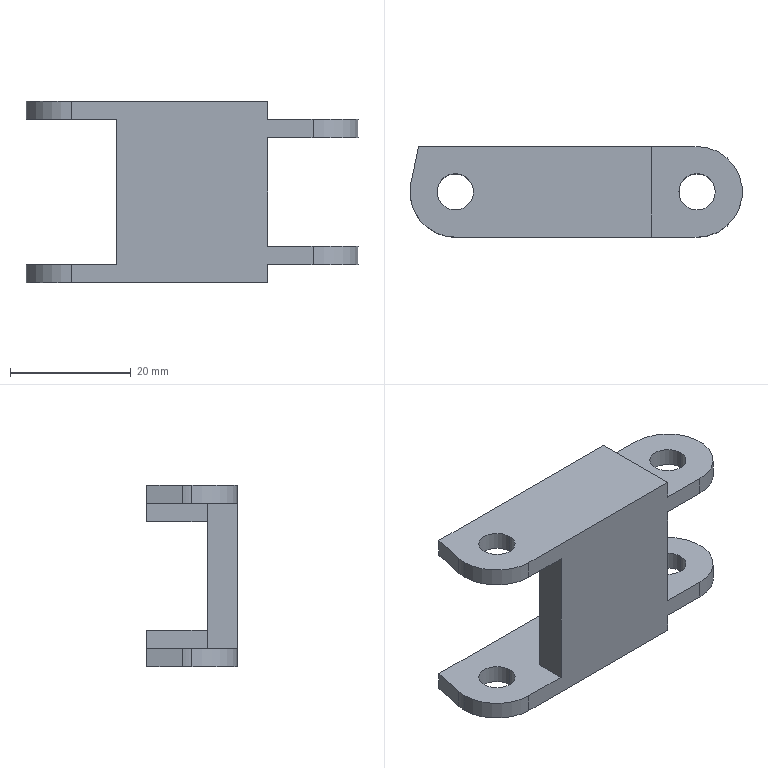Part | SolidWorks | features ICE 3, Extrusion 1 | 1 solid | 34 faces | box 55 x 15 x 30 mm | volume 7665 mm3 | plane 20 | cylinder 14 | commonest cylinder face diameters 6 x8 15 x6
STEP:
#1=CARTESIAN_POINT('',(12.262,7.5,3.));
#2=VERTEX_POINT('',#1);
#3=CARTESIAN_POINT('',(6.262,7.5,3.));
#4=VERTEX_POINT('',#3);
#5=CARTESIAN_POINT('',(9.262,7.5,3.));
#6=DIRECTION('',(0.,0.,-1.));
#7=DIRECTION('',(-1.,0.,0.));
#8=AXIS2_PLACEMENT_3D('',#5,#6,#7);
#9=CIRCLE('',#8,3.);
#10=EDGE_CURVE('',#2,#4,#9,.T.);
#11=ORIENTED_EDGE('',*,*,#10,.F.);
#12=CARTESIAN_POINT('',(12.262,7.5,0.));
#13=VERTEX_POINT('',#12);
#14=CARTESIAN_POINT('',(12.262,7.5,30.));
#15=DIRECTION('',(0.,0.,-1.));
#16=VECTOR('',#15,1000.);
#17=LINE('',#14,#16);
#18=EDGE_CURVE('',#2,#13,#17,.T.);
#19=ORIENTED_EDGE('',*,*,#18,.T.);
#20=CARTESIAN_POINT('',(6.262,7.5,0.));
#21=VERTEX_POINT('',#20);
#22=CARTESIAN_POINT('',(9.262,7.5,0.));
#23=DIRECTION('',(0.,0.,1.));
#24=DIRECTION('',(1.,0.,0.));
#25=AXIS2_PLACEMENT_3D('',#22,#23,#24);
#26=CIRCLE('',#25,3.);
#27=EDGE_CURVE('',#21,#13,#26,.T.);
#28=ORIENTED_EDGE('',*,*,#27,.F.);
#29=CARTESIAN_POINT('',(6.262,7.5,30.));
#30=DIRECTION('',(0.,0.,-1.));
#31=VECTOR('',#30,1000.);
#32=LINE('',#29,#31);
#33=EDGE_CURVE('',#4,#21,#32,.T.);
#34=ORIENTED_EDGE('',*,*,#33,.F.);
#35=EDGE_LOOP('',(#11,#19,#28,#34));
#36=FACE_OUTER_BOUND('',#35,.T.);
#37=CARTESIAN_POINT('',(9.262,7.5,30.));
#38=DIRECTION('',(0.,0.,-1.));
#39=DIRECTION('',(-1.,0.,0.));
#40=AXIS2_PLACEMENT_3D('',#37,#38,#39);
#41=CYLINDRICAL_SURFACE('',#40,3.);
#42=ADVANCED_FACE('',(#36),#41,.F.);
#43=CARTESIAN_POINT('',(9.262,0.,3.));
#44=VERTEX_POINT('',#43);
#45=CARTESIAN_POINT('',(1.762,7.5,3.));
#46=VERTEX_POINT('',#45);
#47=CARTESIAN_POINT('',(9.262,7.5,3.));
#48=DIRECTION('',(0.,0.,-1.));
#49=DIRECTION('',(-1.,0.,0.));
#50=AXIS2_PLACEMENT_3D('',#47,#48,#49);
#51=CIRCLE('',#50,7.5);
#52=EDGE_CURVE('',#44,#46,#51,.T.);
#53=ORIENTED_EDGE('',*,*,#52,.T.);
#54=CARTESIAN_POINT('',(1.762,7.5,0.));
#55=VERTEX_POINT('',#54);
#56=CARTESIAN_POINT('',(1.762,7.5,30.));
#57=DIRECTION('',(0.,0.,-1.));
#58=VECTOR('',#57,1000.);
#59=LINE('',#56,#58);
#60=EDGE_CURVE('',#46,#55,#59,.T.);
#61=ORIENTED_EDGE('',*,*,#60,.T.);
#62=CARTESIAN_POINT('',(9.262,0.,0.));
#63=VERTEX_POINT('',#62);
#64=CARTESIAN_POINT('',(9.262,7.5,0.));
#65=DIRECTION('',(0.,0.,1.));
#66=DIRECTION('',(1.,0.,0.));
#67=AXIS2_PLACEMENT_3D('',#64,#65,#66);
#68=CIRCLE('',#67,7.5);
#69=EDGE_CURVE('',#55,#63,#68,.T.);
#70=ORIENTED_EDGE('',*,*,#69,.T.);
#71=CARTESIAN_POINT('',(9.262,0.,30.));
#72=DIRECTION('',(0.,0.,-1.));
#73=VECTOR('',#72,1000.);
#74=LINE('',#71,#73);
#75=EDGE_CURVE('',#44,#63,#74,.T.);
#76=ORIENTED_EDGE('',*,*,#75,.F.);
#77=EDGE_LOOP('',(#53,#61,#70,#76));
#78=FACE_OUTER_BOUND('',#77,.T.);
#79=CARTESIAN_POINT('',(9.262,7.5,30.));
#80=DIRECTION('',(0.,0.,-1.));
#81=DIRECTION('',(-1.,0.,0.));
#82=AXIS2_PLACEMENT_3D('',#79,#80,#81);
#83=CYLINDRICAL_SURFACE('',#82,7.5);
#84=ADVANCED_FACE('',(#78),#83,.T.);
#85=CARTESIAN_POINT('',(6.262,7.5,30.));
#86=VERTEX_POINT('',#85);
#87=CARTESIAN_POINT('',(12.262,7.5,30.));
#88=VERTEX_POINT('',#87);
#89=CARTESIAN_POINT('',(9.262,7.5,30.));
#90=DIRECTION('',(0.,0.,1.));
#91=DIRECTION('',(1.,0.,0.));
#92=AXIS2_PLACEMENT_3D('',#89,#90,#91);
#93=CIRCLE('',#92,3.);
#94=EDGE_CURVE('',#86,#88,#93,.T.);
#95=ORIENTED_EDGE('',*,*,#94,.T.);
#96=CARTESIAN_POINT('',(12.262,7.5,27.));
#97=VERTEX_POINT('',#96);
#98=CARTESIAN_POINT('',(12.262,7.5,30.));
#99=DIRECTION('',(0.,0.,-1.));
#100=VECTOR('',#99,1000.);
#101=LINE('',#98,#100);
#102=EDGE_CURVE('',#88,#97,#101,.T.);
#103=ORIENTED_EDGE('',*,*,#102,.T.);
#104=CARTESIAN_POINT('',(6.262,7.5,27.));
#105=VERTEX_POINT('',#104);
#106=CARTESIAN_POINT('',(9.262,7.5,27.));
#107=DIRECTION('',(0.,0.,1.));
#108=DIRECTION('',(1.,0.,0.));
#109=AXIS2_PLACEMENT_3D('',#106,#107,#108);
#110=CIRCLE('',#109,3.);
#111=EDGE_CURVE('',#105,#97,#110,.T.);
#112=ORIENTED_EDGE('',*,*,#111,.F.);
#113=CARTESIAN_POINT('',(6.262,7.5,30.));
#114=DIRECTION('',(0.,0.,-1.));
#115=VECTOR('',#114,1000.);
#116=LINE('',#113,#115);
#117=EDGE_CURVE('',#86,#105,#116,.T.);
#118=ORIENTED_EDGE('',*,*,#117,.F.);
#119=EDGE_LOOP('',(#95,#103,#112,#118));
#120=FACE_OUTER_BOUND('',#119,.T.);
#121=CARTESIAN_POINT('',(9.262,7.5,30.));
#122=DIRECTION('',(0.,0.,-1.));
#123=DIRECTION('',(-1.,0.,0.));
#124=AXIS2_PLACEMENT_3D('',#121,#122,#123);
#125=CYLINDRICAL_SURFACE('',#124,3.);
#126=ADVANCED_FACE('',(#120),#125,.F.);
#127=CARTESIAN_POINT('',(1.762,7.5,30.));
#128=VERTEX_POINT('',#127);
#129=CARTESIAN_POINT('',(9.262,0.,30.));
#130=VERTEX_POINT('',#129);
#131=CARTESIAN_POINT('',(9.262,7.5,30.));
#132=DIRECTION('',(0.,0.,1.));
#133=DIRECTION('',(1.,0.,0.));
#134=AXIS2_PLACEMENT_3D('',#131,#132,#133);
#135=CIRCLE('',#134,7.5);
#136=EDGE_CURVE('',#128,#130,#135,.T.);
#137=ORIENTED_EDGE('',*,*,#136,.F.);
#138=CARTESIAN_POINT('',(1.762,7.5,27.));
#139=VERTEX_POINT('',#138);
#140=CARTESIAN_POINT('',(1.762,7.5,30.));
#141=DIRECTION('',(0.,0.,-1.));
#142=VECTOR('',#141,1000.);
#143=LINE('',#140,#142);
#144=EDGE_CURVE('',#128,#139,#143,.T.);
#145=ORIENTED_EDGE('',*,*,#144,.T.);
#146=CARTESIAN_POINT('',(9.262,0.,27.));
#147=VERTEX_POINT('',#146);
#148=CARTESIAN_POINT('',(9.262,7.5,27.));
#149=DIRECTION('',(0.,0.,1.));
#150=DIRECTION('',(1.,0.,0.));
#151=AXIS2_PLACEMENT_3D('',#148,#149,#150);
#152=CIRCLE('',#151,7.5);
#153=EDGE_CURVE('',#139,#147,#152,.T.);
#154=ORIENTED_EDGE('',*,*,#153,.T.);
#155=CARTESIAN_POINT('',(9.262,0.,30.));
#156=DIRECTION('',(0.,0.,-1.));
#157=VECTOR('',#156,1000.);
#158=LINE('',#155,#157);
#159=EDGE_CURVE('',#130,#147,#158,.T.);
#160=ORIENTED_EDGE('',*,*,#159,.F.);
#161=EDGE_LOOP('',(#137,#145,#154,#160));
#162=FACE_OUTER_BOUND('',#161,.T.);
#163=CARTESIAN_POINT('',(9.262,7.5,30.));
#164=DIRECTION('',(0.,0.,-1.));
#165=DIRECTION('',(-1.,0.,0.));
#166=AXIS2_PLACEMENT_3D('',#163,#164,#165);
#167=CYLINDRICAL_SURFACE('',#166,7.5);
#168=ADVANCED_FACE('',(#162),#167,.T.);
#169=CARTESIAN_POINT('',(52.262,7.5,27.));
#170=VERTEX_POINT('',#169);
#171=CARTESIAN_POINT('',(46.262,7.5,27.));
#172=VERTEX_POINT('',#171);
#173=CARTESIAN_POINT('',(49.262,7.5,27.));
#174=DIRECTION('',(0.,0.,-1.));
#175=DIRECTION('',(-1.,0.,0.));
#176=AXIS2_PLACEMENT_3D('',#173,#174,#175);
#177=CIRCLE('',#176,3.);
#178=EDGE_CURVE('',#170,#172,#177,.T.);
#179=ORIENTED_EDGE('',*,*,#178,.F.);
#180=CARTESIAN_POINT('',(52.262,7.5,24.));
#181=VERTEX_POINT('',#180);
#182=CARTESIAN_POINT('',(52.262,7.5,30.));
#183=DIRECTION('',(0.,0.,-1.));
#184=VECTOR('',#183,1000.);
#185=LINE('',#182,#184);
#186=EDGE_CURVE('',#170,#181,#185,.T.);
#187=ORIENTED_EDGE('',*,*,#186,.T.);
#188=CARTESIAN_POINT('',(46.262,7.5,24.));
#189=VERTEX_POINT('',#188);
#190=CARTESIAN_POINT('',(49.262,7.5,24.));
#191=DIRECTION('',(0.,0.,1.));
#192=DIRECTION('',(1.,0.,0.));
#193=AXIS2_PLACEMENT_3D('',#190,#191,#192);
#194=CIRCLE('',#193,3.);
#195=EDGE_CURVE('',#189,#181,#194,.T.);
#196=ORIENTED_EDGE('',*,*,#195,.F.);
#197=CARTESIAN_POINT('',(46.262,7.5,30.));
#198=DIRECTION('',(0.,0.,-1.));
#199=VECTOR('',#198,1000.);
#200=LINE('',#197,#199);
#201=EDGE_CURVE('',#172,#189,#200,.T.);
#202=ORIENTED_EDGE('',*,*,#201,.F.);
#203=EDGE_LOOP('',(#179,#187,#196,#202));
#204=FACE_OUTER_BOUND('',#203,.T.);
#205=CARTESIAN_POINT('',(49.262,7.5,30.));
#206=DIRECTION('',(0.,0.,-1.));
#207=DIRECTION('',(-1.,0.,0.));
#208=AXIS2_PLACEMENT_3D('',#205,#206,#207);
#209=CYLINDRICAL_SURFACE('',#208,3.);
#210=ADVANCED_FACE('',(#204),#209,.F.);
#211=CARTESIAN_POINT('',(52.262,7.5,6.));
#212=VERTEX_POINT('',#211);
#213=CARTESIAN_POINT('',(46.262,7.5,6.));
#214=VERTEX_POINT('',#213);
#215=CARTESIAN_POINT('',(49.262,7.5,6.));
#216=DIRECTION('',(0.,0.,-1.));
#217=DIRECTION('',(-1.,0.,0.));
#218=AXIS2_PLACEMENT_3D('',#215,#216,#217);
#219=CIRCLE('',#218,3.);
#220=EDGE_CURVE('',#212,#214,#219,.T.);
#221=ORIENTED_EDGE('',*,*,#220,.F.);
#222=CARTESIAN_POINT('',(52.262,7.5,3.));
#223=VERTEX_POINT('',#222);
#224=CARTESIAN_POINT('',(52.262,7.5,30.));
#225=DIRECTION('',(0.,0.,-1.));
#226=VECTOR('',#225,1000.);
#227=LINE('',#224,#226);
#228=EDGE_CURVE('',#212,#223,#227,.T.);
#229=ORIENTED_EDGE('',*,*,#228,.T.);
#230=CARTESIAN_POINT('',(46.262,7.5,3.));
#231=VERTEX_POINT('',#230);
#232=CARTESIAN_POINT('',(49.262,7.5,3.));
#233=DIRECTION('',(0.,0.,1.));
#234=DIRECTION('',(1.,0.,0.));
#235=AXIS2_PLACEMENT_3D('',#232,#233,#234);
#236=CIRCLE('',#235,3.);
#237=EDGE_CURVE('',#231,#223,#236,.T.);
#238=ORIENTED_EDGE('',*,*,#237,.F.);
#239=CARTESIAN_POINT('',(46.262,7.5,30.));
#240=DIRECTION('',(0.,0.,-1.));
#241=VECTOR('',#240,1000.);
#242=LINE('',#239,#241);
#243=EDGE_CURVE('',#214,#231,#242,.T.);
#244=ORIENTED_EDGE('',*,*,#243,.F.);
#245=EDGE_LOOP('',(#221,#229,#238,#244));
#246=FACE_OUTER_BOUND('',#245,.T.);
#247=CARTESIAN_POINT('',(49.262,7.5,30.));
#248=DIRECTION('',(0.,0.,-1.));
#249=DIRECTION('',(-1.,0.,0.));
#250=AXIS2_PLACEMENT_3D('',#247,#248,#249);
#251=CYLINDRICAL_SURFACE('',#250,3.);
#252=ADVANCED_FACE('',(#246),#251,.F.);
#253=ORIENTED_EDGE('',*,*,#228,.F.);
#254=CARTESIAN_POINT('',(49.262,7.5,6.));
#255=DIRECTION('',(0.,0.,-1.));
#256=DIRECTION('',(-1.,0.,0.));
#257=AXIS2_PLACEMENT_3D('',#254,#255,#256);
#258=CIRCLE('',#257,3.);
#259=EDGE_CURVE('',#214,#212,#258,.T.);
#260=ORIENTED_EDGE('',*,*,#259,.F.);
#261=ORIENTED_EDGE('',*,*,#243,.T.);
#262=CARTESIAN_POINT('',(49.262,7.5,3.));
#263=DIRECTION('',(0.,0.,1.));
#264=DIRECTION('',(1.,0.,0.));
#265=AXIS2_PLACEMENT_3D('',#262,#263,#264);
#266=CIRCLE('',#265,3.);
#267=EDGE_CURVE('',#223,#231,#266,.T.);
#268=ORIENTED_EDGE('',*,*,#267,.F.);
#269=EDGE_LOOP('',(#253,#260,#261,#268));
#270=FACE_OUTER_BOUND('',#269,.T.);
#271=CARTESIAN_POINT('',(49.262,7.5,30.));
#272=DIRECTION('',(0.,0.,-1.));
#273=DIRECTION('',(-1.,0.,0.));
#274=AXIS2_PLACEMENT_3D('',#271,#272,#273);
#275=CYLINDRICAL_SURFACE('',#274,3.);
#276=ADVANCED_FACE('',(#270),#275,.F.);
#277=CARTESIAN_POINT('',(49.262,15.,6.));
#278=VERTEX_POINT('',#277);
#279=CARTESIAN_POINT('',(49.262,0.,6.));
#280=VERTEX_POINT('',#279);
#281=CARTESIAN_POINT('',(49.262,7.5,6.));
#282=DIRECTION('',(0.,0.,-1.));
#283=DIRECTION('',(-1.,0.,0.));
#284=AXIS2_PLACEMENT_3D('',#281,#282,#283);
#285=CIRCLE('',#284,7.5);
#286=EDGE_CURVE('',#278,#280,#285,.T.);
#287=ORIENTED_EDGE('',*,*,#286,.T.);
#288=CARTESIAN_POINT('',(49.262,0.,3.));
#289=VERTEX_POINT('',#288);
#290=CARTESIAN_POINT('',(49.262,0.,30.));
#291=DIRECTION('',(0.,0.,-1.));
#292=VECTOR('',#291,1000.);
#293=LINE('',#290,#292);
#294=EDGE_CURVE('',#280,#289,#293,.T.);
#295=ORIENTED_EDGE('',*,*,#294,.T.);
#296=CARTESIAN_POINT('',(49.262,15.,3.));
#297=VERTEX_POINT('',#296);
#298=CARTESIAN_POINT('',(49.262,7.5,3.));
#299=DIRECTION('',(0.,0.,1.));
#300=DIRECTION('',(1.,0.,0.));
#301=AXIS2_PLACEMENT_3D('',#298,#299,#300);
#302=CIRCLE('',#301,7.5);
#303=EDGE_CURVE('',#289,#297,#302,.T.);
#304=ORIENTED_EDGE('',*,*,#303,.T.);
#305=CARTESIAN_POINT('',(49.262,15.,30.));
#306=DIRECTION('',(0.,0.,-1.));
#307=VECTOR('',#306,1000.);
#308=LINE('',#305,#307);
#309=EDGE_CURVE('',#278,#297,#308,.T.);
#310=ORIENTED_EDGE('',*,*,#309,.F.);
#311=EDGE_LOOP('',(#287,#295,#304,#310));
#312=FACE_OUTER_BOUND('',#311,.T.);
#313=CARTESIAN_POINT('',(49.262,7.5,30.));
#314=DIRECTION('',(0.,0.,-1.));
#315=DIRECTION('',(-1.,0.,0.));
#316=AXIS2_PLACEMENT_3D('',#313,#314,#315);
#317=CYLINDRICAL_SURFACE('',#316,7.5);
#318=ADVANCED_FACE('',(#312),#317,.T.);
#319=CARTESIAN_POINT('',(36.762,15.,3.));
#320=VERTEX_POINT('',#319);
#321=CARTESIAN_POINT('',(3.188,15.,3.));
#322=VERTEX_POINT('',#321);
#323=CARTESIAN_POINT('',(-13.238,15.,3.));
#324=DIRECTION('',(-1.,0.,0.));
#325=VECTOR('',#324,1000.);
#326=LINE('',#323,#325);
#327=EDGE_CURVE('',#320,#322,#326,.T.);
#328=ORIENTED_EDGE('',*,*,#327,.F.);
#329=CARTESIAN_POINT('',(36.762,15.,6.));
#330=VERTEX_POINT('',#329);
#331=CARTESIAN_POINT('',(36.762,15.,3.));
#332=DIRECTION('',(0.,0.,-1.));
#333=VECTOR('',#332,1000.);
#334=LINE('',#331,#333);
#335=EDGE_CURVE('',#330,#320,#334,.T.);
#336=ORIENTED_EDGE('',*,*,#335,.F.);
#337=CARTESIAN_POINT('',(36.762,15.,6.));
#338=DIRECTION('',(-1.,0.,0.));
#339=VECTOR('',#338,1000.);
#340=LINE('',#337,#339);
#341=EDGE_CURVE('',#278,#330,#340,.T.);
#342=ORIENTED_EDGE('',*,*,#341,.F.);
#343=ORIENTED_EDGE('',*,*,#309,.T.);
#344=CARTESIAN_POINT('',(41.762,15.,3.));
#345=VERTEX_POINT('',#344);
#346=CARTESIAN_POINT('',(41.762,15.,3.));
#347=DIRECTION('',(1.,0.,0.));
#348=VECTOR('',#347,1000.);
#349=LINE('',#346,#348);
#350=EDGE_CURVE('',#345,#297,#349,.T.);
#351=ORIENTED_EDGE('',*,*,#350,.F.);
#352=CARTESIAN_POINT('',(41.762,15.,0.));
#353=VERTEX_POINT('',#352);
#354=CARTESIAN_POINT('',(41.762,15.,-3.));
#355=DIRECTION('',(0.,0.,1.));
#356=VECTOR('',#355,1000.);
#357=LINE('',#354,#356);
#358=EDGE_CURVE('',#353,#345,#357,.T.);
#359=ORIENTED_EDGE('',*,*,#358,.F.);
#360=CARTESIAN_POINT('',(3.188,15.,0.));
#361=VERTEX_POINT('',#360);
#362=CARTESIAN_POINT('',(3.188,15.,0.));
#363=DIRECTION('',(-1.,0.,0.));
#364=VECTOR('',#363,1000.);
#365=LINE('',#362,#364);
#366=EDGE_CURVE('',#353,#361,#365,.T.);
#367=ORIENTED_EDGE('',*,*,#366,.T.);
#368=CARTESIAN_POINT('',(3.188,15.,30.));
#369=DIRECTION('',(0.,0.,-1.));
#370=VECTOR('',#369,1000.);
#371=LINE('',#368,#370);
#372=EDGE_CURVE('',#322,#361,#371,.T.);
#373=ORIENTED_EDGE('',*,*,#372,.F.);
#374=EDGE_LOOP('',(#328,#336,#342,#343,#351,#359,#367,#373));
#375=FACE_OUTER_BOUND('',#374,.T.);
#376=CARTESIAN_POINT('',(3.188,15.,30.));
#377=DIRECTION('',(0.,-1.,0.));
#378=DIRECTION('',(0.,0.,-1.));
#379=AXIS2_PLACEMENT_3D('',#376,#377,#378);
#380=PLANE('',#379);
#381=ADVANCED_FACE('',(#375),#380,.F.);
#382=CARTESIAN_POINT('',(16.762,5.,3.));
#383=VERTEX_POINT('',#382);
#384=CARTESIAN_POINT('',(16.762,5.,27.));
#385=VERTEX_POINT('',#384);
#386=CARTESIAN_POINT('',(16.762,5.,3.));
#387=DIRECTION('',(0.,0.,1.));
#388=VECTOR('',#387,1000.);
#389=LINE('',#386,#388);
#390=EDGE_CURVE('',#383,#385,#389,.T.);
#391=ORIENTED_EDGE('',*,*,#390,.F.);
#392=CARTESIAN_POINT('',(16.762,0.,3.));
#393=VERTEX_POINT('',#392);
#394=CARTESIAN_POINT('',(16.762,-15.,3.));
#395=DIRECTION('',(0.,1.,0.));
#396=VECTOR('',#395,1000.);
#397=LINE('',#394,#396);
#398=EDGE_CURVE('',#393,#383,#397,.T.);
#399=ORIENTED_EDGE('',*,*,#398,.F.);
#400=CARTESIAN_POINT('',(16.762,0.,27.));
#401=VERTEX_POINT('',#400);
#402=CARTESIAN_POINT('',(16.762,0.,30.));
#403=DIRECTION('',(0.,0.,-1.));
#404=VECTOR('',#403,1000.);
#405=LINE('',#402,#404);
#406=EDGE_CURVE('',#401,#393,#405,.T.);
#407=ORIENTED_EDGE('',*,*,#406,.F.);
#408=CARTESIAN_POINT('',(16.762,-15.,27.));
#409=DIRECTION('',(0.,1.,0.));
#410=VECTOR('',#409,1000.);
#411=LINE('',#408,#410);
#412=EDGE_CURVE('',#401,#385,#411,.T.);
#413=ORIENTED_EDGE('',*,*,#412,.T.);
#414=EDGE_LOOP('',(#391,#399,#407,#413));
#415=FACE_OUTER_BOUND('',#414,.T.);
#416=CARTESIAN_POINT('',(16.762,-15.,3.));
#417=DIRECTION('',(1.,0.,0.));
#418=DIRECTION('',(0.,0.,-1.));
#419=AXIS2_PLACEMENT_3D('',#416,#417,#418);
#420=PLANE('',#419);
#421=ADVANCED_FACE('',(#415),#420,.F.);
#422=ORIENTED_EDGE('',*,*,#186,.F.);
#423=CARTESIAN_POINT('',(49.262,7.5,27.));
#424=DIRECTION('',(0.,0.,-1.));
#425=DIRECTION('',(-1.,0.,0.));
#426=AXIS2_PLACEMENT_3D('',#423,#424,#425);
#427=CIRCLE('',#426,3.);
#428=EDGE_CURVE('',#172,#170,#427,.T.);
#429=ORIENTED_EDGE('',*,*,#428,.F.);
#430=ORIENTED_EDGE('',*,*,#201,.T.);
#431=CARTESIAN_POINT('',(49.262,7.5,24.));
#432=DIRECTION('',(0.,0.,1.));
#433=DIRECTION('',(1.,0.,0.));
#434=AXIS2_PLACEMENT_3D('',#431,#432,#433);
#435=CIRCLE('',#434,3.);
#436=EDGE_CURVE('',#181,#189,#435,.T.);
#437=ORIENTED_EDGE('',*,*,#436,.F.);
#438=EDGE_LOOP('',(#422,#429,#430,#437));
#439=FACE_OUTER_BOUND('',#438,.T.);
#440=CARTESIAN_POINT('',(49.262,7.5,30.));
#441=DIRECTION('',(0.,0.,-1.));
#442=DIRECTION('',(-1.,0.,0.));
#443=AXIS2_PLACEMENT_3D('',#440,#441,#442);
#444=CYLINDRICAL_SURFACE('',#443,3.);
#445=ADVANCED_FACE('',(#439),#444,.F.);
#446=CARTESIAN_POINT('',(3.188,15.,30.));
#447=VERTEX_POINT('',#446);
#448=CARTESIAN_POINT('',(3.188,15.,27.));
#449=VERTEX_POINT('',#448);
#450=CARTESIAN_POINT('',(3.188,15.,30.));
#451=DIRECTION('',(0.,0.,-1.));
#452=VECTOR('',#451,1000.);
#453=LINE('',#450,#452);
#454=EDGE_CURVE('',#447,#449,#453,.T.);
#455=ORIENTED_EDGE('',*,*,#454,.T.);
#456=CARTESIAN_POINT('',(1.926,9.059,27.));
#457=VERTEX_POINT('',#456);
#458=CARTESIAN_POINT('',(1.926,9.059,27.));
#459=DIRECTION('',(-0.2079,-0.9781,0.));
#460=VECTOR('',#459,1000.);
#461=LINE('',#458,#460);
#462=EDGE_CURVE('',#449,#457,#461,.T.);
#463=ORIENTED_EDGE('',*,*,#462,.T.);
#464=CARTESIAN_POINT('',(1.926,9.059,30.));
#465=VERTEX_POINT('',#464);
#466=CARTESIAN_POINT('',(1.926,9.059,30.));
#467=DIRECTION('',(0.,0.,-1.));
#468=VECTOR('',#467,1000.);
#469=LINE('',#466,#468);
#470=EDGE_CURVE('',#465,#457,#469,.T.);
#471=ORIENTED_EDGE('',*,*,#470,.F.);
#472=CARTESIAN_POINT('',(1.926,9.059,30.));
#473=DIRECTION('',(-0.2079,-0.9781,0.));
#474=VECTOR('',#473,1000.);
#475=LINE('',#472,#474);
#476=EDGE_CURVE('',#447,#465,#475,.T.);
#477=ORIENTED_EDGE('',*,*,#476,.F.);
#478=EDGE_LOOP('',(#455,#463,#471,#477));
#479=FACE_OUTER_BOUND('',#478,.T.);
#480=CARTESIAN_POINT('',(1.926,9.059,30.));
#481=DIRECTION('',(0.9781,-0.2079,0.));
#482=DIRECTION('',(0.2079,0.9781,0.));
#483=AXIS2_PLACEMENT_3D('',#480,#481,#482);
#484=PLANE('',#483);
#485=ADVANCED_FACE('',(#479),#484,.F.);
#486=ORIENTED_EDGE('',*,*,#144,.F.);
#487=CARTESIAN_POINT('',(9.262,7.5,30.));
#488=DIRECTION('',(0.,0.,1.));
#489=DIRECTION('',(1.,0.,0.));
#490=AXIS2_PLACEMENT_3D('',#487,#488,#489);
#491=CIRCLE('',#490,7.5);
#492=EDGE_CURVE('',#465,#128,#491,.T.);
#493=ORIENTED_EDGE('',*,*,#492,.F.);
#494=ORIENTED_EDGE('',*,*,#470,.T.);
#495=CARTESIAN_POINT('',(9.262,7.5,27.));
#496=DIRECTION('',(0.,0.,1.));
#497=DIRECTION('',(1.,0.,0.));
#498=AXIS2_PLACEMENT_3D('',#495,#496,#497);
#499=CIRCLE('',#498,7.5);
#500=EDGE_CURVE('',#457,#139,#499,.T.);
#501=ORIENTED_EDGE('',*,*,#500,.T.);
#502=EDGE_LOOP('',(#486,#493,#494,#501));
#503=FACE_OUTER_BOUND('',#502,.T.);
#504=CARTESIAN_POINT('',(9.262,7.5,30.));
#505=DIRECTION('',(0.,0.,-1.));
#506=DIRECTION('',(-1.,0.,0.));
#507=AXIS2_PLACEMENT_3D('',#504,#505,#506);
#508=CYLINDRICAL_SURFACE('',#507,7.5);
#509=ADVANCED_FACE('',(#503),#508,.T.);
#510=ORIENTED_EDGE('',*,*,#102,.F.);
#511=CARTESIAN_POINT('',(9.262,7.5,30.));
#512=DIRECTION('',(0.,0.,1.));
#513=DIRECTION('',(1.,0.,0.));
#514=AXIS2_PLACEMENT_3D('',#511,#512,#513);
#515=CIRCLE('',#514,3.);
#516=EDGE_CURVE('',#88,#86,#515,.T.);
#517=ORIENTED_EDGE('',*,*,#516,.T.);
#518=ORIENTED_EDGE('',*,*,#117,.T.);
#519=CARTESIAN_POINT('',(9.262,7.5,27.));
#520=DIRECTION('',(0.,0.,1.));
#521=DIRECTION('',(1.,0.,0.));
#522=AXIS2_PLACEMENT_3D('',#519,#520,#521);
#523=CIRCLE('',#522,3.);
#524=EDGE_CURVE('',#97,#105,#523,.T.);
#525=ORIENTED_EDGE('',*,*,#524,.F.);
#526=EDGE_LOOP('',(#510,#517,#518,#525));
#527=FACE_OUTER_BOUND('',#526,.T.);
#528=CARTESIAN_POINT('',(9.262,7.5,30.));
#529=DIRECTION('',(0.,0.,-1.));
#530=DIRECTION('',(-1.,0.,0.));
#531=AXIS2_PLACEMENT_3D('',#528,#529,#530);
#532=CYLINDRICAL_SURFACE('',#531,3.);
#533=ADVANCED_FACE('',(#527),#532,.F.);
#534=CARTESIAN_POINT('',(41.762,15.,30.));
#535=VERTEX_POINT('',#534);
#536=CARTESIAN_POINT('',(41.762,0.,30.));
#537=VERTEX_POINT('',#536);
#538=CARTESIAN_POINT('',(41.762,7.5,30.));
#539=DIRECTION('',(0.,-1.,0.));
#540=VECTOR('',#539,1000.);
#541=LINE('',#538,#540);
#542=EDGE_CURVE('',#535,#537,#541,.T.);
#543=ORIENTED_EDGE('',*,*,#542,.F.);
#544=CARTESIAN_POINT('',(3.188,15.,30.));
#545=DIRECTION('',(-1.,0.,0.));
#546=VECTOR('',#545,1000.);
#547=LINE('',#544,#546);
#548=EDGE_CURVE('',#535,#447,#547,.T.);
#549=ORIENTED_EDGE('',*,*,#548,.T.);
#550=ORIENTED_EDGE('',*,*,#476,.T.);
#551=ORIENTED_EDGE('',*,*,#492,.T.);
#552=ORIENTED_EDGE('',*,*,#136,.T.);
#553=CARTESIAN_POINT('',(49.262,0.,30.));
#554=DIRECTION('',(1.,0.,0.));
#555=VECTOR('',#554,1000.);
#556=LINE('',#553,#555);
#557=EDGE_CURVE('',#130,#537,#556,.T.);
#558=ORIENTED_EDGE('',*,*,#557,.T.);
#559=EDGE_LOOP('',(#543,#549,#550,#551,#552,#558));
#560=FACE_OUTER_BOUND('',#559,.T.);
#561=ORIENTED_EDGE('',*,*,#94,.F.);
#562=ORIENTED_EDGE('',*,*,#516,.F.);
#563=EDGE_LOOP('',(#561,#562));
#564=FACE_BOUND('',#563,.T.);
#565=CARTESIAN_POINT('',(49.262,7.5,30.));
#566=DIRECTION('',(0.,0.,1.));
#567=DIRECTION('',(1.,0.,0.));
#568=AXIS2_PLACEMENT_3D('',#565,#566,#567);
#569=PLANE('',#568);
#570=ADVANCED_FACE('',(#560,#564),#569,.T.);
#571=ORIENTED_EDGE('',*,*,#366,.F.);
#572=CARTESIAN_POINT('',(41.762,0.,0.));
#573=VERTEX_POINT('',#572);
#574=CARTESIAN_POINT('',(41.762,7.5,0.));
#575=DIRECTION('',(0.,-1.,0.));
#576=VECTOR('',#575,1000.);
#577=LINE('',#574,#576);
#578=EDGE_CURVE('',#353,#573,#577,.T.);
#579=ORIENTED_EDGE('',*,*,#578,.T.);
#580=CARTESIAN_POINT('',(49.262,0.,0.));
#581=DIRECTION('',(1.,0.,0.));
#582=VECTOR('',#581,1000.);
#583=LINE('',#580,#582);
#584=EDGE_CURVE('',#63,#573,#583,.T.);
#585=ORIENTED_EDGE('',*,*,#584,.F.);
#586=ORIENTED_EDGE('',*,*,#69,.F.);
#587=CARTESIAN_POINT('',(1.926,9.059,0.));
#588=VERTEX_POINT('',#587);
#589=CARTESIAN_POINT('',(9.262,7.5,0.));
#590=DIRECTION('',(0.,0.,1.));
#591=DIRECTION('',(1.,0.,0.));
#592=AXIS2_PLACEMENT_3D('',#589,#590,#591);
#593=CIRCLE('',#592,7.5);
#594=EDGE_CURVE('',#588,#55,#593,.T.);
#595=ORIENTED_EDGE('',*,*,#594,.F.);
#596=CARTESIAN_POINT('',(1.926,9.059,0.));
#597=DIRECTION('',(-0.2079,-0.9781,0.));
#598=VECTOR('',#597,1000.);
#599=LINE('',#596,#598);
#600=EDGE_CURVE('',#361,#588,#599,.T.);
#601=ORIENTED_EDGE('',*,*,#600,.F.);
#602=EDGE_LOOP('',(#571,#579,#585,#586,#595,#601));
#603=FACE_OUTER_BOUND('',#602,.T.);
#604=ORIENTED_EDGE('',*,*,#27,.T.);
#605=CARTESIAN_POINT('',(9.262,7.5,0.));
#606=DIRECTION('',(0.,0.,1.));
#607=DIRECTION('',(1.,0.,0.));
#608=AXIS2_PLACEMENT_3D('',#605,#606,#607);
#609=CIRCLE('',#608,3.);
#610=EDGE_CURVE('',#13,#21,#609,.T.);
#611=ORIENTED_EDGE('',*,*,#610,.T.);
#612=EDGE_LOOP('',(#604,#611));
#613=FACE_BOUND('',#612,.T.);
#614=CARTESIAN_POINT('',(49.262,7.5,0.));
#615=DIRECTION('',(0.,0.,1.));
#616=DIRECTION('',(1.,0.,0.));
#617=AXIS2_PLACEMENT_3D('',#614,#615,#616);
#618=PLANE('',#617);
#619=ADVANCED_FACE('',(#603,#613),#618,.F.);
#620=CARTESIAN_POINT('',(36.762,15.,27.));
#621=VERTEX_POINT('',#620);
#622=CARTESIAN_POINT('',(36.762,15.,24.));
#623=VERTEX_POINT('',#622);
#624=CARTESIAN_POINT('',(36.762,15.,24.));
#625=DIRECTION('',(0.,0.,-1.));
#626=VECTOR('',#625,1000.);
#627=LINE('',#624,#626);
#628=EDGE_CURVE('',#621,#623,#627,.T.);
#629=ORIENTED_EDGE('',*,*,#628,.F.);
#630=CARTESIAN_POINT('',(-13.238,15.,27.));
#631=DIRECTION('',(1.,0.,0.));
#632=VECTOR('',#631,1000.);
#633=LINE('',#630,#632);
#634=EDGE_CURVE('',#449,#621,#633,.T.);
#635=ORIENTED_EDGE('',*,*,#634,.F.);
#636=ORIENTED_EDGE('',*,*,#454,.F.);
#637=ORIENTED_EDGE('',*,*,#548,.F.);
#638=CARTESIAN_POINT('',(41.762,15.,27.));
#639=VERTEX_POINT('',#638);
#640=CARTESIAN_POINT('',(41.762,15.,27.));
#641=DIRECTION('',(0.,0.,1.));
#642=VECTOR('',#641,1000.);
#643=LINE('',#640,#642);
#644=EDGE_CURVE('',#639,#535,#643,.T.);
#645=ORIENTED_EDGE('',*,*,#644,.F.);
#646=CARTESIAN_POINT('',(49.262,15.,27.));
#647=VERTEX_POINT('',#646);
#648=CARTESIAN_POINT('',(41.762,15.,27.));
#649=DIRECTION('',(-1.,0.,0.));
#650=VECTOR('',#649,1000.);
#651=LINE('',#648,#650);
#652=EDGE_CURVE('',#647,#639,#651,.T.);
#653=ORIENTED_EDGE('',*,*,#652,.F.);
#654=CARTESIAN_POINT('',(49.262,15.,24.));
#655=VERTEX_POINT('',#654);
#656=CARTESIAN_POINT('',(49.262,15.,30.));
#657=DIRECTION('',(0.,0.,-1.));
#658=VECTOR('',#657,1000.);
#659=LINE('',#656,#658);
#660=EDGE_CURVE('',#647,#655,#659,.T.);
#661=ORIENTED_EDGE('',*,*,#660,.T.);
#662=CARTESIAN_POINT('',(36.762,15.,24.));
#663=DIRECTION('',(1.,0.,0.));
#664=VECTOR('',#663,1000.);
#665=LINE('',#662,#664);
#666=EDGE_CURVE('',#623,#655,#665,.T.);
#667=ORIENTED_EDGE('',*,*,#666,.F.);
#668=EDGE_LOOP('',(#629,#635,#636,#637,#645,#653,#661,#667));
#669=FACE_OUTER_BOUND('',#668,.T.);
#670=CARTESIAN_POINT('',(3.188,15.,30.));
#671=DIRECTION('',(0.,-1.,0.));
#672=DIRECTION('',(0.,0.,-1.));
#673=AXIS2_PLACEMENT_3D('',#670,#671,#672);
#674=PLANE('',#673);
#675=ADVANCED_FACE('',(#669),#674,.F.);
#676=CARTESIAN_POINT('',(1.926,9.059,3.));
#677=VERTEX_POINT('',#676);
#678=CARTESIAN_POINT('',(1.926,9.059,30.));
#679=DIRECTION('',(0.,0.,-1.));
#680=VECTOR('',#679,1000.);
#681=LINE('',#678,#680);
#682=EDGE_CURVE('',#677,#588,#681,.T.);
#683=ORIENTED_EDGE('',*,*,#682,.F.);
#684=CARTESIAN_POINT('',(1.926,9.059,3.));
#685=DIRECTION('',(0.2079,0.9781,0.));
#686=VECTOR('',#685,1000.);
#687=LINE('',#684,#686);
#688=EDGE_CURVE('',#677,#322,#687,.T.);
#689=ORIENTED_EDGE('',*,*,#688,.T.);
#690=ORIENTED_EDGE('',*,*,#372,.T.);
#691=ORIENTED_EDGE('',*,*,#600,.T.);
#692=EDGE_LOOP('',(#683,#689,#690,#691));
#693=FACE_OUTER_BOUND('',#692,.T.);
#694=CARTESIAN_POINT('',(1.926,9.059,30.));
#695=DIRECTION('',(0.9781,-0.2079,0.));
#696=DIRECTION('',(0.2079,0.9781,0.));
#697=AXIS2_PLACEMENT_3D('',#694,#695,#696);
#698=PLANE('',#697);
#699=ADVANCED_FACE('',(#693),#698,.F.);
#700=ORIENTED_EDGE('',*,*,#60,.F.);
#701=CARTESIAN_POINT('',(9.262,7.5,3.));
#702=DIRECTION('',(0.,0.,-1.));
#703=DIRECTION('',(-1.,0.,0.));
#704=AXIS2_PLACEMENT_3D('',#701,#702,#703);
#705=CIRCLE('',#704,7.5);
#706=EDGE_CURVE('',#46,#677,#705,.T.);
#707=ORIENTED_EDGE('',*,*,#706,.T.);
#708=ORIENTED_EDGE('',*,*,#682,.T.);
#709=ORIENTED_EDGE('',*,*,#594,.T.);
#710=EDGE_LOOP('',(#700,#707,#708,#709));
#711=FACE_OUTER_BOUND('',#710,.T.);
#712=CARTESIAN_POINT('',(9.262,7.5,30.));
#713=DIRECTION('',(0.,0.,-1.));
#714=DIRECTION('',(-1.,0.,0.));
#715=AXIS2_PLACEMENT_3D('',#712,#713,#714);
#716=CYLINDRICAL_SURFACE('',#715,7.5);
#717=ADVANCED_FACE('',(#711),#716,.T.);
#718=ORIENTED_EDGE('',*,*,#294,.F.);
#719=CARTESIAN_POINT('',(41.762,0.,6.));
#720=VERTEX_POINT('',#719);
#721=CARTESIAN_POINT('',(49.262,0.,6.));
#722=DIRECTION('',(-1.,0.,0.));
#723=VECTOR('',#722,1000.);
#724=LINE('',#721,#723);
#725=EDGE_CURVE('',#280,#720,#724,.T.);
#726=ORIENTED_EDGE('',*,*,#725,.T.);
#727=CARTESIAN_POINT('',(41.762,0.,24.));
#728=VERTEX_POINT('',#727);
#729=CARTESIAN_POINT('',(41.762,0.,30.));
#730=DIRECTION('',(0.,0.,1.));
#731=VECTOR('',#730,1000.);
#732=LINE('',#729,#731);
#733=EDGE_CURVE('',#720,#728,#732,.T.);
#734=ORIENTED_EDGE('',*,*,#733,.T.);
#735=CARTESIAN_POINT('',(49.262,0.,24.));
#736=VERTEX_POINT('',#735);
#737=CARTESIAN_POINT('',(49.262,0.,24.));
#738=DIRECTION('',(1.,0.,0.));
#739=VECTOR('',#738,1000.);
#740=LINE('',#737,#739);
#741=EDGE_CURVE('',#728,#736,#740,.T.);
#742=ORIENTED_EDGE('',*,*,#741,.T.);
#743=CARTESIAN_POINT('',(49.262,0.,27.));
#744=VERTEX_POINT('',#743);
#745=CARTESIAN_POINT('',(49.262,0.,30.));
#746=DIRECTION('',(0.,0.,-1.));
#747=VECTOR('',#746,1000.);
#748=LINE('',#745,#747);
#749=EDGE_CURVE('',#744,#736,#748,.T.);
#750=ORIENTED_EDGE('',*,*,#749,.F.);
#751=CARTESIAN_POINT('',(41.762,0.,27.));
#752=VERTEX_POINT('',#751);
#753=CARTESIAN_POINT('',(49.262,0.,27.));
#754=DIRECTION('',(-1.,0.,0.));
#755=VECTOR('',#754,1000.);
#756=LINE('',#753,#755);
#757=EDGE_CURVE('',#744,#752,#756,.T.);
#758=ORIENTED_EDGE('',*,*,#757,.T.);
#759=CARTESIAN_POINT('',(41.762,0.,30.));
#760=DIRECTION('',(0.,0.,1.));
#761=VECTOR('',#760,1000.);
#762=LINE('',#759,#761);
#763=EDGE_CURVE('',#752,#537,#762,.T.);
#764=ORIENTED_EDGE('',*,*,#763,.T.);
#765=ORIENTED_EDGE('',*,*,#557,.F.);
#766=ORIENTED_EDGE('',*,*,#159,.T.);
#767=CARTESIAN_POINT('',(49.262,0.,27.));
#768=DIRECTION('',(1.,0.,0.));
#769=VECTOR('',#768,1000.);
#770=LINE('',#767,#769);
#771=EDGE_CURVE('',#147,#401,#770,.T.);
#772=ORIENTED_EDGE('',*,*,#771,.T.);
#773=ORIENTED_EDGE('',*,*,#406,.T.);
#774=CARTESIAN_POINT('',(49.262,0.,3.));
#775=DIRECTION('',(-1.,0.,0.));
#776=VECTOR('',#775,1000.);
#777=LINE('',#774,#776);
#778=EDGE_CURVE('',#393,#44,#777,.T.);
#779=ORIENTED_EDGE('',*,*,#778,.T.);
#780=ORIENTED_EDGE('',*,*,#75,.T.);
#781=ORIENTED_EDGE('',*,*,#584,.T.);
#782=CARTESIAN_POINT('',(41.762,0.,3.));
#783=VERTEX_POINT('',#782);
#784=CARTESIAN_POINT('',(41.762,0.,30.));
#785=DIRECTION('',(0.,0.,1.));
#786=VECTOR('',#785,1000.);
#787=LINE('',#784,#786);
#788=EDGE_CURVE('',#573,#783,#787,.T.);
#789=ORIENTED_EDGE('',*,*,#788,.T.);
#790=CARTESIAN_POINT('',(49.262,0.,3.));
#791=DIRECTION('',(1.,0.,0.));
#792=VECTOR('',#791,1000.);
#793=LINE('',#790,#792);
#794=EDGE_CURVE('',#783,#289,#793,.T.);
#795=ORIENTED_EDGE('',*,*,#794,.T.);
#796=EDGE_LOOP('',(#718,#726,#734,#742,#750,#758,#764,#765,#766,#772,#773,#779,#780,#781,#789,#795));
#797=FACE_OUTER_BOUND('',#796,.T.);
#798=CARTESIAN_POINT('',(49.262,0.,30.));
#799=DIRECTION('',(0.,1.,0.));
#800=DIRECTION('',(-1.,0.,0.));
#801=AXIS2_PLACEMENT_3D('',#798,#799,#800);
#802=PLANE('',#801);
#803=ADVANCED_FACE('',(#797),#802,.F.);
#804=ORIENTED_EDGE('',*,*,#749,.T.);
#805=CARTESIAN_POINT('',(49.262,7.5,24.));
#806=DIRECTION('',(0.,0.,1.));
#807=DIRECTION('',(1.,0.,0.));
#808=AXIS2_PLACEMENT_3D('',#805,#806,#807);
#809=CIRCLE('',#808,7.5);
#810=EDGE_CURVE('',#736,#655,#809,.T.);
#811=ORIENTED_EDGE('',*,*,#810,.T.);
#812=ORIENTED_EDGE('',*,*,#660,.F.);
#813=CARTESIAN_POINT('',(49.262,7.5,27.));
#814=DIRECTION('',(0.,0.,-1.));
#815=DIRECTION('',(-1.,0.,0.));
#816=AXIS2_PLACEMENT_3D('',#813,#814,#815);
#817=CIRCLE('',#816,7.5);
#818=EDGE_CURVE('',#647,#744,#817,.T.);
#819=ORIENTED_EDGE('',*,*,#818,.T.);
#820=EDGE_LOOP('',(#804,#811,#812,#819));
#821=FACE_OUTER_BOUND('',#820,.T.);
#822=CARTESIAN_POINT('',(49.262,7.5,30.));
#823=DIRECTION('',(0.,0.,-1.));
#824=DIRECTION('',(-1.,0.,0.));
#825=AXIS2_PLACEMENT_3D('',#822,#823,#824);
#826=CYLINDRICAL_SURFACE('',#825,7.5);
#827=ADVANCED_FACE('',(#821),#826,.T.);
#828=ORIENTED_EDGE('',*,*,#18,.F.);
#829=CARTESIAN_POINT('',(9.262,7.5,3.));
#830=DIRECTION('',(0.,0.,-1.));
#831=DIRECTION('',(-1.,0.,0.));
#832=AXIS2_PLACEMENT_3D('',#829,#830,#831);
#833=CIRCLE('',#832,3.);
#834=EDGE_CURVE('',#4,#2,#833,.T.);
#835=ORIENTED_EDGE('',*,*,#834,.F.);
#836=ORIENTED_EDGE('',*,*,#33,.T.);
#837=ORIENTED_EDGE('',*,*,#610,.F.);
#838=EDGE_LOOP('',(#828,#835,#836,#837));
#839=FACE_OUTER_BOUND('',#838,.T.);
#840=CARTESIAN_POINT('',(9.262,7.5,30.));
#841=DIRECTION('',(0.,0.,-1.));
#842=DIRECTION('',(-1.,0.,0.));
#843=AXIS2_PLACEMENT_3D('',#840,#841,#842);
#844=CYLINDRICAL_SURFACE('',#843,3.);
#845=ADVANCED_FACE('',(#839),#844,.F.);
#846=ORIENTED_EDGE('',*,*,#428,.T.);
#847=ORIENTED_EDGE('',*,*,#178,.T.);
#848=EDGE_LOOP('',(#846,#847));
#849=FACE_BOUND('',#848,.T.);
#850=ORIENTED_EDGE('',*,*,#818,.F.);
#851=ORIENTED_EDGE('',*,*,#652,.T.);
#852=CARTESIAN_POINT('',(41.762,-15.,27.));
#853=DIRECTION('',(0.,1.,0.));
#854=VECTOR('',#853,1000.);
#855=LINE('',#852,#854);
#856=EDGE_CURVE('',#752,#639,#855,.T.);
#857=ORIENTED_EDGE('',*,*,#856,.F.);
#858=ORIENTED_EDGE('',*,*,#757,.F.);
#859=EDGE_LOOP('',(#850,#851,#857,#858));
#860=FACE_OUTER_BOUND('',#859,.T.);
#861=CARTESIAN_POINT('',(41.762,-15.,27.));
#862=DIRECTION('',(0.,0.,-1.));
#863=DIRECTION('',(-1.,0.,0.));
#864=AXIS2_PLACEMENT_3D('',#861,#862,#863);
#865=PLANE('',#864);
#866=ADVANCED_FACE('',(#849,#860),#865,.F.);
#867=ORIENTED_EDGE('',*,*,#542,.T.);
#868=ORIENTED_EDGE('',*,*,#763,.F.);
#869=ORIENTED_EDGE('',*,*,#856,.T.);
#870=ORIENTED_EDGE('',*,*,#644,.T.);
#871=EDGE_LOOP('',(#867,#868,#869,#870));
#872=FACE_OUTER_BOUND('',#871,.T.);
#873=CARTESIAN_POINT('',(41.762,-15.,27.));
#874=DIRECTION('',(-1.,0.,0.));
#875=DIRECTION('',(0.,0.,1.));
#876=AXIS2_PLACEMENT_3D('',#873,#874,#875);
#877=PLANE('',#876);
#878=ADVANCED_FACE('',(#872),#877,.F.);
#879=ORIENTED_EDGE('',*,*,#358,.T.);
#880=CARTESIAN_POINT('',(41.762,-15.,3.));
#881=DIRECTION('',(0.,1.,0.));
#882=VECTOR('',#881,1000.);
#883=LINE('',#880,#882);
#884=EDGE_CURVE('',#783,#345,#883,.T.);
#885=ORIENTED_EDGE('',*,*,#884,.F.);
#886=ORIENTED_EDGE('',*,*,#788,.F.);
#887=ORIENTED_EDGE('',*,*,#578,.F.);
#888=EDGE_LOOP('',(#879,#885,#886,#887));
#889=FACE_OUTER_BOUND('',#888,.T.);
#890=CARTESIAN_POINT('',(41.762,-15.,-3.));
#891=DIRECTION('',(-1.,0.,0.));
#892=DIRECTION('',(0.,0.,1.));
#893=AXIS2_PLACEMENT_3D('',#890,#891,#892);
#894=PLANE('',#893);
#895=ADVANCED_FACE('',(#889),#894,.F.);
#896=ORIENTED_EDGE('',*,*,#237,.T.);
#897=ORIENTED_EDGE('',*,*,#267,.T.);
#898=EDGE_LOOP('',(#896,#897));
#899=FACE_BOUND('',#898,.T.);
#900=ORIENTED_EDGE('',*,*,#884,.T.);
#901=ORIENTED_EDGE('',*,*,#350,.T.);
#902=ORIENTED_EDGE('',*,*,#303,.F.);
#903=ORIENTED_EDGE('',*,*,#794,.F.);
#904=EDGE_LOOP('',(#900,#901,#902,#903));
#905=FACE_OUTER_BOUND('',#904,.T.);
#906=CARTESIAN_POINT('',(41.762,-15.,3.));
#907=DIRECTION('',(0.,0.,1.));
#908=DIRECTION('',(1.,0.,0.));
#909=AXIS2_PLACEMENT_3D('',#906,#907,#908);
#910=PLANE('',#909);
#911=ADVANCED_FACE('',(#899,#905),#910,.F.);
#912=ORIENTED_EDGE('',*,*,#111,.T.);
#913=ORIENTED_EDGE('',*,*,#524,.T.);
#914=EDGE_LOOP('',(#912,#913));
#915=FACE_BOUND('',#914,.T.);
#916=ORIENTED_EDGE('',*,*,#634,.T.);
#917=CARTESIAN_POINT('',(36.762,5.,27.));
#918=VERTEX_POINT('',#917);
#919=CARTESIAN_POINT('',(36.762,5.,27.));
#920=DIRECTION('',(0.,1.,0.));
#921=VECTOR('',#920,1000.);
#922=LINE('',#919,#921);
#923=EDGE_CURVE('',#918,#621,#922,.T.);
#924=ORIENTED_EDGE('',*,*,#923,.F.);
#925=CARTESIAN_POINT('',(-3.238,5.,27.));
#926=DIRECTION('',(1.,0.,0.));
#927=VECTOR('',#926,1000.);
#928=LINE('',#925,#927);
#929=EDGE_CURVE('',#385,#918,#928,.T.);
#930=ORIENTED_EDGE('',*,*,#929,.F.);
#931=ORIENTED_EDGE('',*,*,#412,.F.);
#932=ORIENTED_EDGE('',*,*,#771,.F.);
#933=ORIENTED_EDGE('',*,*,#153,.F.);
#934=ORIENTED_EDGE('',*,*,#500,.F.);
#935=ORIENTED_EDGE('',*,*,#462,.F.);
#936=EDGE_LOOP('',(#916,#924,#930,#931,#932,#933,#934,#935));
#937=FACE_OUTER_BOUND('',#936,.T.);
#938=CARTESIAN_POINT('',(-13.238,-15.,27.));
#939=DIRECTION('',(0.,0.,1.));
#940=DIRECTION('',(1.,0.,0.));
#941=AXIS2_PLACEMENT_3D('',#938,#939,#940);
#942=PLANE('',#941);
#943=ADVANCED_FACE('',(#915,#937),#942,.F.);
#944=ORIENTED_EDGE('',*,*,#834,.T.);
#945=ORIENTED_EDGE('',*,*,#10,.T.);
#946=EDGE_LOOP('',(#944,#945));
#947=FACE_BOUND('',#946,.T.);
#948=ORIENTED_EDGE('',*,*,#688,.F.);
#949=ORIENTED_EDGE('',*,*,#706,.F.);
#950=ORIENTED_EDGE('',*,*,#52,.F.);
#951=ORIENTED_EDGE('',*,*,#778,.F.);
#952=ORIENTED_EDGE('',*,*,#398,.T.);
#953=CARTESIAN_POINT('',(36.762,5.,3.));
#954=VERTEX_POINT('',#953);
#955=CARTESIAN_POINT('',(-3.238,5.,3.));
#956=DIRECTION('',(-1.,0.,0.));
#957=VECTOR('',#956,1000.);
#958=LINE('',#955,#957);
#959=EDGE_CURVE('',#954,#383,#958,.T.);
#960=ORIENTED_EDGE('',*,*,#959,.F.);
#961=CARTESIAN_POINT('',(36.762,5.,3.));
#962=DIRECTION('',(0.,1.,0.));
#963=VECTOR('',#962,1000.);
#964=LINE('',#961,#963);
#965=EDGE_CURVE('',#954,#320,#964,.T.);
#966=ORIENTED_EDGE('',*,*,#965,.T.);
#967=ORIENTED_EDGE('',*,*,#327,.T.);
#968=EDGE_LOOP('',(#948,#949,#950,#951,#952,#960,#966,#967));
#969=FACE_OUTER_BOUND('',#968,.T.);
#970=CARTESIAN_POINT('',(-13.238,-15.,3.));
#971=DIRECTION('',(0.,0.,-1.));
#972=DIRECTION('',(-1.,0.,0.));
#973=AXIS2_PLACEMENT_3D('',#970,#971,#972);
#974=PLANE('',#973);
#975=ADVANCED_FACE('',(#947,#969),#974,.F.);
#976=ORIENTED_EDGE('',*,*,#259,.T.);
#977=ORIENTED_EDGE('',*,*,#220,.T.);
#978=EDGE_LOOP('',(#976,#977));
#979=FACE_BOUND('',#978,.T.);
#980=ORIENTED_EDGE('',*,*,#341,.T.);
#981=CARTESIAN_POINT('',(36.762,5.,6.));
#982=VERTEX_POINT('',#981);
#983=CARTESIAN_POINT('',(36.762,5.,6.));
#984=DIRECTION('',(0.,1.,0.));
#985=VECTOR('',#984,1000.);
#986=LINE('',#983,#985);
#987=EDGE_CURVE('',#982,#330,#986,.T.);
#988=ORIENTED_EDGE('',*,*,#987,.F.);
#989=CARTESIAN_POINT('',(41.762,5.,6.));
#990=VERTEX_POINT('',#989);
#991=CARTESIAN_POINT('',(36.762,5.,6.));
#992=DIRECTION('',(-1.,0.,0.));
#993=VECTOR('',#992,1000.);
#994=LINE('',#991,#993);
#995=EDGE_CURVE('',#990,#982,#994,.T.);
#996=ORIENTED_EDGE('',*,*,#995,.F.);
#997=CARTESIAN_POINT('',(41.762,-7.,6.));
#998=DIRECTION('',(0.,1.,0.));
#999=VECTOR('',#998,1000.);
#1000=LINE('',#997,#999);
#1001=EDGE_CURVE('',#720,#990,#1000,.T.);
#1002=ORIENTED_EDGE('',*,*,#1001,.F.);
#1003=ORIENTED_EDGE('',*,*,#725,.F.);
#1004=ORIENTED_EDGE('',*,*,#286,.F.);
#1005=EDGE_LOOP('',(#980,#988,#996,#1002,#1003,#1004));
#1006=FACE_OUTER_BOUND('',#1005,.T.);
#1007=CARTESIAN_POINT('',(36.762,5.,6.));
#1008=DIRECTION('',(0.,0.,-1.));
#1009=DIRECTION('',(-1.,0.,0.));
#1010=AXIS2_PLACEMENT_3D('',#1007,#1008,#1009);
#1011=PLANE('',#1010);
#1012=ADVANCED_FACE('',(#979,#1006),#1011,.F.);
#1013=ORIENTED_EDGE('',*,*,#810,.F.);
#1014=ORIENTED_EDGE('',*,*,#741,.F.);
#1015=CARTESIAN_POINT('',(41.762,5.,24.));
#1016=VERTEX_POINT('',#1015);
#1017=CARTESIAN_POINT('',(41.762,-7.,24.));
#1018=DIRECTION('',(0.,1.,0.));
#1019=VECTOR('',#1018,1000.);
#1020=LINE('',#1017,#1019);
#1021=EDGE_CURVE('',#728,#1016,#1020,.T.);
#1022=ORIENTED_EDGE('',*,*,#1021,.T.);
#1023=CARTESIAN_POINT('',(36.762,5.,24.));
#1024=VERTEX_POINT('',#1023);
#1025=CARTESIAN_POINT('',(36.762,5.,24.));
#1026=DIRECTION('',(1.,0.,0.));
#1027=VECTOR('',#1026,1000.);
#1028=LINE('',#1025,#1027);
#1029=EDGE_CURVE('',#1024,#1016,#1028,.T.);
#1030=ORIENTED_EDGE('',*,*,#1029,.F.);
#1031=CARTESIAN_POINT('',(36.762,5.,24.));
#1032=DIRECTION('',(0.,1.,0.));
#1033=VECTOR('',#1032,1000.);
#1034=LINE('',#1031,#1033);
#1035=EDGE_CURVE('',#1024,#623,#1034,.T.);
#1036=ORIENTED_EDGE('',*,*,#1035,.T.);
#1037=ORIENTED_EDGE('',*,*,#666,.T.);
#1038=EDGE_LOOP('',(#1013,#1014,#1022,#1030,#1036,#1037));
#1039=FACE_OUTER_BOUND('',#1038,.T.);
#1040=ORIENTED_EDGE('',*,*,#195,.T.);
#1041=ORIENTED_EDGE('',*,*,#436,.T.);
#1042=EDGE_LOOP('',(#1040,#1041));
#1043=FACE_BOUND('',#1042,.T.);
#1044=CARTESIAN_POINT('',(36.762,5.,24.));
#1045=DIRECTION('',(0.,0.,1.));
#1046=DIRECTION('',(1.,0.,0.));
#1047=AXIS2_PLACEMENT_3D('',#1044,#1045,#1046);
#1048=PLANE('',#1047);
#1049=ADVANCED_FACE('',(#1039,#1043),#1048,.F.);
#1050=CARTESIAN_POINT('',(41.762,5.,24.));
#1051=DIRECTION('',(0.,0.,1.));
#1052=VECTOR('',#1051,1000.);
#1053=LINE('',#1050,#1052);
#1054=EDGE_CURVE('',#990,#1016,#1053,.T.);
#1055=ORIENTED_EDGE('',*,*,#1054,.F.);
#1056=ORIENTED_EDGE('',*,*,#995,.T.);
#1057=CARTESIAN_POINT('',(36.762,5.,3.));
#1058=DIRECTION('',(0.,0.,-1.));
#1059=VECTOR('',#1058,1000.);
#1060=LINE('',#1057,#1059);
#1061=EDGE_CURVE('',#982,#954,#1060,.T.);
#1062=ORIENTED_EDGE('',*,*,#1061,.T.);
#1063=ORIENTED_EDGE('',*,*,#959,.T.);
#1064=ORIENTED_EDGE('',*,*,#390,.T.);
#1065=ORIENTED_EDGE('',*,*,#929,.T.);
#1066=CARTESIAN_POINT('',(36.762,5.,24.));
#1067=DIRECTION('',(0.,0.,-1.));
#1068=VECTOR('',#1067,1000.);
#1069=LINE('',#1066,#1068);
#1070=EDGE_CURVE('',#918,#1024,#1069,.T.);
#1071=ORIENTED_EDGE('',*,*,#1070,.T.);
#1072=ORIENTED_EDGE('',*,*,#1029,.T.);
#1073=EDGE_LOOP('',(#1055,#1056,#1062,#1063,#1064,#1065,#1071,#1072));
#1074=FACE_OUTER_BOUND('',#1073,.T.);
#1075=CARTESIAN_POINT('',(0.,5.,0.));
#1076=DIRECTION('',(0.,1.,0.));
#1077=DIRECTION('',(0.,0.,1.));
#1078=AXIS2_PLACEMENT_3D('',#1075,#1076,#1077);
#1079=PLANE('',#1078);
#1080=ADVANCED_FACE('',(#1074),#1079,.T.);
#1081=ORIENTED_EDGE('',*,*,#628,.T.);
#1082=ORIENTED_EDGE('',*,*,#1035,.F.);
#1083=ORIENTED_EDGE('',*,*,#1070,.F.);
#1084=ORIENTED_EDGE('',*,*,#923,.T.);
#1085=EDGE_LOOP('',(#1081,#1082,#1083,#1084));
#1086=FACE_OUTER_BOUND('',#1085,.T.);
#1087=CARTESIAN_POINT('',(36.762,5.,24.));
#1088=DIRECTION('',(1.,0.,0.));
#1089=DIRECTION('',(0.,0.,-1.));
#1090=AXIS2_PLACEMENT_3D('',#1087,#1088,#1089);
#1091=PLANE('',#1090);
#1092=ADVANCED_FACE('',(#1086),#1091,.F.);
#1093=ORIENTED_EDGE('',*,*,#335,.T.);
#1094=ORIENTED_EDGE('',*,*,#965,.F.);
#1095=ORIENTED_EDGE('',*,*,#1061,.F.);
#1096=ORIENTED_EDGE('',*,*,#987,.T.);
#1097=EDGE_LOOP('',(#1093,#1094,#1095,#1096));
#1098=FACE_OUTER_BOUND('',#1097,.T.);
#1099=CARTESIAN_POINT('',(36.762,5.,3.));
#1100=DIRECTION('',(1.,0.,0.));
#1101=DIRECTION('',(0.,0.,-1.));
#1102=AXIS2_PLACEMENT_3D('',#1099,#1100,#1101);
#1103=PLANE('',#1102);
#1104=ADVANCED_FACE('',(#1098),#1103,.F.);
#1105=ORIENTED_EDGE('',*,*,#1001,.T.);
#1106=ORIENTED_EDGE('',*,*,#1054,.T.);
#1107=ORIENTED_EDGE('',*,*,#1021,.F.);
#1108=ORIENTED_EDGE('',*,*,#733,.F.);
#1109=EDGE_LOOP('',(#1105,#1106,#1107,#1108));
#1110=FACE_OUTER_BOUND('',#1109,.T.);
#1111=CARTESIAN_POINT('',(41.762,-7.,24.));
#1112=DIRECTION('',(-1.,0.,0.));
#1113=DIRECTION('',(0.,0.,1.));
#1114=AXIS2_PLACEMENT_3D('',#1111,#1112,#1113);
#1115=PLANE('',#1114);
#1116=ADVANCED_FACE('',(#1110),#1115,.F.);
#1117=CLOSED_SHELL('',(#42,#84,#126,#168,#210,#252,#276,#318,#381,#421,#445,#485,#509,#533,#570,#619,#675,#699,#717,#803,#827,#845,#866,#878,#895,#911,#943,#975,#1012,#1049,#1080,#1092,#1104,#1116));
#1118=MANIFOLD_SOLID_BREP('',#1117);
#1119=CARTESIAN_POINT('',(0.,0.,0.));
#1120=DIRECTION('',(0.,0.,1.));
#1121=DIRECTION('',(1.,0.,0.));
#1122=AXIS2_PLACEMENT_3D('',#1119,#1120,#1121);
#1123=(LENGTH_UNIT()NAMED_UNIT(*)SI_UNIT(.MILLI.,.METRE.));
#1124=UNCERTAINTY_MEASURE_WITH_UNIT(LENGTH_MEASURE(0.00001),#1123,'','');
#1125=(NAMED_UNIT(*)PLANE_ANGLE_UNIT()SI_UNIT($,.RADIAN.));
#1126=(NAMED_UNIT(*)SI_UNIT($,.STERADIAN.)SOLID_ANGLE_UNIT());
#1127=(GEOMETRIC_REPRESENTATION_CONTEXT(3)GLOBAL_UNCERTAINTY_ASSIGNED_CONTEXT((#1124))GLOBAL_UNIT_ASSIGNED_CONTEXT((#1123,#1125,#1126))REPRESENTATION_CONTEXT('',''));
#1128=ADVANCED_BREP_SHAPE_REPRESENTATION('',(#1118,#1122),#1127);